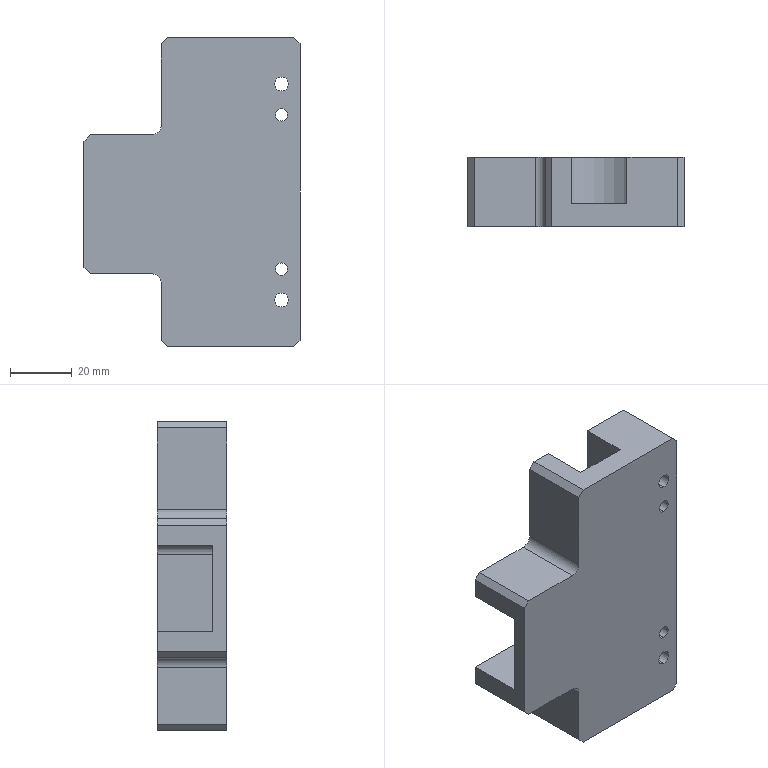Part | STEP file | PN_0049 | 1 solid | 83 faces | box 70 x 22.5 x 100 mm | volume 72311 mm3 | cylinder 36 | plane 27 | cone 20 | commonest cylinder face diameters 2.5 x20 4 x4 4.5 x4 8 x4 6 x3 28 x1